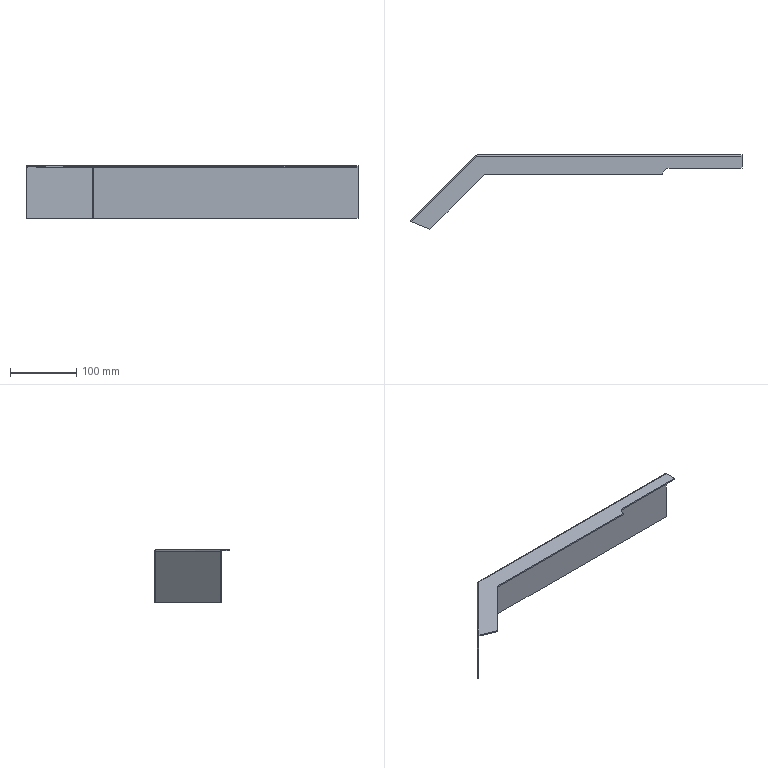Part | STEP file | Left Side Plate Filler Piece | 1 solid | 24 faces | box 502.056 x 112.482 x 80 mm | volume 112790 mm3 | plane 16 | cylinder 5 | spline 3 | commonest cylinder face diameters 1 x2 5 x2 20 x1
STEP:
#1=CARTESIAN_POINT('',(193.538,20.962,-2.5));
#2=VERTEX_POINT('',#1);
#3=CARTESIAN_POINT('',(-207.092,20.962,-2.5));
#4=VERTEX_POINT('',#3);
#5=CARTESIAN_POINT('',(0.,20.962,-2.5));
#6=DIRECTION('',(-1.,0.,0.));
#7=VECTOR('',#6,1000.);
#8=LINE('',#5,#7);
#9=EDGE_CURVE('',#2,#4,#8,.T.);
#10=ORIENTED_EDGE('',*,*,#9,.F.);
#11=CARTESIAN_POINT('',(193.538,20.962,-80.));
#12=VERTEX_POINT('',#11);
#13=CARTESIAN_POINT('',(193.538,20.962,0.));
#14=DIRECTION('',(0.,0.,1.));
#15=VECTOR('',#14,1000.);
#16=LINE('',#13,#15);
#17=EDGE_CURVE('',#12,#2,#16,.T.);
#18=ORIENTED_EDGE('',*,*,#17,.F.);
#19=CARTESIAN_POINT('',(-207.092,20.962,-80.));
#20=VERTEX_POINT('',#19);
#21=CARTESIAN_POINT('',(0.,20.962,-80.));
#22=DIRECTION('',(1.,0.,0.));
#23=VECTOR('',#22,1000.);
#24=LINE('',#21,#23);
#25=EDGE_CURVE('',#20,#12,#24,.T.);
#26=ORIENTED_EDGE('',*,*,#25,.F.);
#27=CARTESIAN_POINT('',(-207.092,20.962,0.));
#28=DIRECTION('',(0.,0.,-1.));
#29=VECTOR('',#28,1000.);
#30=LINE('',#27,#29);
#31=EDGE_CURVE('',#4,#20,#30,.T.);
#32=ORIENTED_EDGE('',*,*,#31,.F.);
#33=EDGE_LOOP('',(#10,#18,#26,#32));
#34=FACE_OUTER_BOUND('',#33,.T.);
#35=CARTESIAN_POINT('',(0.,20.962,0.));
#36=DIRECTION('',(0.,-1.,0.));
#37=DIRECTION('',(0.,0.,-1.));
#38=AXIS2_PLACEMENT_3D('',#35,#36,#37);
#39=PLANE('',#38);
#40=ADVANCED_FACE('',(#34),#39,.F.);
#41=CARTESIAN_POINT('',(-207.092,18.962,-80.));
#42=VERTEX_POINT('',#41);
#43=CARTESIAN_POINT('',(-207.092,18.962,-2.5));
#44=VERTEX_POINT('',#43);
#45=CARTESIAN_POINT('',(-207.092,18.962,-2.));
#46=DIRECTION('',(0.,0.,1.));
#47=VECTOR('',#46,1000.);
#48=LINE('',#45,#47);
#49=EDGE_CURVE('',#42,#44,#48,.T.);
#50=ORIENTED_EDGE('',*,*,#49,.T.);
#51=CARTESIAN_POINT('',(-207.092,18.962,-2.5));
#52=DIRECTION('',(0.,1.,0.));
#53=VECTOR('',#52,1000.);
#54=LINE('',#51,#53);
#55=EDGE_CURVE('',#44,#4,#54,.T.);
#56=ORIENTED_EDGE('',*,*,#55,.T.);
#57=ORIENTED_EDGE('',*,*,#31,.T.);
#58=CARTESIAN_POINT('',(-207.092,18.962,-80.));
#59=DIRECTION('',(0.,-1.,0.));
#60=VECTOR('',#59,1000.);
#61=LINE('',#58,#60);
#62=EDGE_CURVE('',#20,#42,#61,.T.);
#63=ORIENTED_EDGE('',*,*,#62,.T.);
#64=EDGE_LOOP('',(#50,#56,#57,#63));
#65=FACE_OUTER_BOUND('',#64,.T.);
#66=CARTESIAN_POINT('',(-207.092,18.962,-2.));
#67=DIRECTION('',(-1.,0.,0.));
#68=DIRECTION('',(0.,0.,1.));
#69=AXIS2_PLACEMENT_3D('',#66,#67,#68);
#70=PLANE('',#69);
#71=ADVANCED_FACE('',(#65),#70,.T.);
#72=ORIENTED_EDGE('',*,*,#9,.T.);
#73=CARTESIAN_POINT('',(-207.426,18.462,0.));
#74=VERTEX_POINT('',#73);
#75=CARTESIAN_POINT('',(-207.092,20.962,-2.5));
#76=CARTESIAN_POINT('',(-207.12,20.962,-2.173));
#77=CARTESIAN_POINT('',(-207.148,20.897,-1.846));
#78=CARTESIAN_POINT('',(-207.204,20.646,-1.241));
#79=CARTESIAN_POINT('',(-207.232,20.461,-0.9636));
#80=CARTESIAN_POINT('',(-207.287,19.998,-0.5008));
#81=CARTESIAN_POINT('',(-207.315,19.721,-0.3155));
#82=CARTESIAN_POINT('',(-207.371,19.116,-0.06507));
#83=CARTESIAN_POINT('',(-207.399,18.789,0.));
#84=CARTESIAN_POINT('',(-207.426,18.462,0.));
#85=B_SPLINE_CURVE_WITH_KNOTS('',3,(#75,#76,#77,#78,#79,#80,#81,#82,#83,#84),.UNSPECIFIED.,.F.,.F.,(4,2,2,2,4),(0.,0.25,0.5,0.75,1.),.UNSPECIFIED.);
#86=EDGE_CURVE('',#4,#74,#85,.T.);
#87=ORIENTED_EDGE('',*,*,#86,.T.);
#88=CARTESIAN_POINT('',(193.538,18.462,0.));
#89=VERTEX_POINT('',#88);
#90=CARTESIAN_POINT('',(193.538,18.462,0.));
#91=DIRECTION('',(1.,0.,0.));
#92=VECTOR('',#91,1000.);
#93=LINE('',#90,#92);
#94=EDGE_CURVE('',#74,#89,#93,.T.);
#95=ORIENTED_EDGE('',*,*,#94,.T.);
#96=CARTESIAN_POINT('',(193.538,18.462,-2.5));
#97=DIRECTION('',(-1.,0.,0.));
#98=DIRECTION('',(0.,0.,-1.));
#99=AXIS2_PLACEMENT_3D('',#96,#97,#98);
#100=CIRCLE('',#99,2.5);
#101=EDGE_CURVE('',#89,#2,#100,.T.);
#102=ORIENTED_EDGE('',*,*,#101,.T.);
#103=EDGE_LOOP('',(#72,#87,#95,#102));
#104=FACE_OUTER_BOUND('',#103,.T.);
#105=CARTESIAN_POINT('',(193.538,18.462,-2.5));
#106=DIRECTION('',(1.,0.,0.));
#107=DIRECTION('',(0.,0.,-1.));
#108=AXIS2_PLACEMENT_3D('',#105,#106,#107);
#109=CYLINDRICAL_SURFACE('',#108,2.5);
#110=ADVANCED_FACE('',(#104),#109,.T.);
#111=CARTESIAN_POINT('',(193.538,18.962,-80.));
#112=VERTEX_POINT('',#111);
#113=CARTESIAN_POINT('',(193.538,18.962,-2.5));
#114=VERTEX_POINT('',#113);
#115=CARTESIAN_POINT('',(193.538,18.962,-80.));
#116=DIRECTION('',(0.,0.,1.));
#117=VECTOR('',#116,1000.);
#118=LINE('',#115,#117);
#119=EDGE_CURVE('',#112,#114,#118,.T.);
#120=ORIENTED_EDGE('',*,*,#119,.F.);
#121=CARTESIAN_POINT('',(193.538,20.962,-80.));
#122=DIRECTION('',(0.,-1.,0.));
#123=VECTOR('',#122,1000.);
#124=LINE('',#121,#123);
#125=EDGE_CURVE('',#12,#112,#124,.T.);
#126=ORIENTED_EDGE('',*,*,#125,.F.);
#127=ORIENTED_EDGE('',*,*,#17,.T.);
#128=ORIENTED_EDGE('',*,*,#101,.F.);
#129=CARTESIAN_POINT('',(193.538,0.9619,0.));
#130=VERTEX_POINT('',#129);
#131=CARTESIAN_POINT('',(193.538,0.,0.));
#132=DIRECTION('',(0.,1.,0.));
#133=VECTOR('',#132,1000.);
#134=LINE('',#131,#133);
#135=EDGE_CURVE('',#130,#89,#134,.T.);
#136=ORIENTED_EDGE('',*,*,#135,.F.);
#137=CARTESIAN_POINT('',(193.538,0.9619,-2.));
#138=VERTEX_POINT('',#137);
#139=CARTESIAN_POINT('',(193.538,0.9619,-2.));
#140=DIRECTION('',(0.,0.,-1.));
#141=VECTOR('',#140,1000.);
#142=LINE('',#139,#141);
#143=EDGE_CURVE('',#130,#138,#142,.T.);
#144=ORIENTED_EDGE('',*,*,#143,.T.);
#145=CARTESIAN_POINT('',(193.538,18.462,-2.));
#146=VERTEX_POINT('',#145);
#147=CARTESIAN_POINT('',(193.538,-9.038,-2.));
#148=DIRECTION('',(0.,1.,0.));
#149=VECTOR('',#148,1000.);
#150=LINE('',#147,#149);
#151=EDGE_CURVE('',#138,#146,#150,.T.);
#152=ORIENTED_EDGE('',*,*,#151,.T.);
#153=CARTESIAN_POINT('',(193.538,18.462,-2.5));
#154=DIRECTION('',(1.,0.,0.));
#155=DIRECTION('',(0.,0.,-1.));
#156=AXIS2_PLACEMENT_3D('',#153,#154,#155);
#157=CIRCLE('',#156,0.5);
#158=EDGE_CURVE('',#114,#146,#157,.T.);
#159=ORIENTED_EDGE('',*,*,#158,.F.);
#160=EDGE_LOOP('',(#120,#126,#127,#128,#136,#144,#152,#159));
#161=FACE_OUTER_BOUND('',#160,.T.);
#162=CARTESIAN_POINT('',(193.538,20.962,-80.));
#163=DIRECTION('',(-1.,0.,0.));
#164=DIRECTION('',(0.,-1.,0.));
#165=AXIS2_PLACEMENT_3D('',#162,#163,#164);
#166=PLANE('',#165);
#167=ADVANCED_FACE('',(#161),#166,.F.);
#168=ORIENTED_EDGE('',*,*,#25,.T.);
#169=ORIENTED_EDGE('',*,*,#125,.T.);
#170=CARTESIAN_POINT('',(-208.462,18.962,-80.));
#171=DIRECTION('',(1.,0.,0.));
#172=VECTOR('',#171,1000.);
#173=LINE('',#170,#172);
#174=EDGE_CURVE('',#42,#112,#173,.T.);
#175=ORIENTED_EDGE('',*,*,#174,.F.);
#176=ORIENTED_EDGE('',*,*,#62,.F.);
#177=EDGE_LOOP('',(#168,#169,#175,#176));
#178=FACE_OUTER_BOUND('',#177,.T.);
#179=CARTESIAN_POINT('',(-208.462,20.962,-80.));
#180=DIRECTION('',(0.,0.,1.));
#181=DIRECTION('',(0.,-1.,0.));
#182=AXIS2_PLACEMENT_3D('',#179,#180,#181);
#183=PLANE('',#182);
#184=ADVANCED_FACE('',(#178),#183,.F.);
#185=CARTESIAN_POINT('',(-207.426,18.462,-2.));
#186=VERTEX_POINT('',#185);
#187=CARTESIAN_POINT('',(-207.092,18.962,-2.5));
#188=CARTESIAN_POINT('',(-207.148,18.962,-2.369));
#189=CARTESIAN_POINT('',(-207.204,18.908,-2.239));
#190=CARTESIAN_POINT('',(-207.315,18.723,-2.054));
#191=CARTESIAN_POINT('',(-207.371,18.593,-2.));
#192=CARTESIAN_POINT('',(-207.426,18.462,-2.));
#193=B_SPLINE_CURVE_WITH_KNOTS('',3,(#187,#188,#189,#190,#191,#192),.UNSPECIFIED.,.F.,.F.,(4,2,4),(0.,0.5,1.),.UNSPECIFIED.);
#194=EDGE_CURVE('',#44,#186,#193,.T.);
#195=ORIENTED_EDGE('',*,*,#194,.T.);
#196=CARTESIAN_POINT('',(-207.426,18.462,-1.));
#197=DIRECTION('',(0.,0.,-1.));
#198=VECTOR('',#197,1000.);
#199=LINE('',#196,#198);
#200=EDGE_CURVE('',#74,#186,#199,.T.);
#201=ORIENTED_EDGE('',*,*,#200,.F.);
#202=ORIENTED_EDGE('',*,*,#86,.F.);
#203=ORIENTED_EDGE('',*,*,#55,.F.);
#204=EDGE_LOOP('',(#195,#201,#202,#203));
#205=FACE_OUTER_BOUND('',#204,.T.);
#206=CARTESIAN_POINT('',(-207.426,18.462,0.02));
#207=CARTESIAN_POINT('',(-207.399,18.792,0.02));
#208=CARTESIAN_POINT('',(-207.371,19.122,-0.04559));
#209=CARTESIAN_POINT('',(-207.315,19.731,-0.2981));
#210=CARTESIAN_POINT('',(-207.287,20.011,-0.4848));
#211=CARTESIAN_POINT('',(-207.232,20.477,-0.9513));
#212=CARTESIAN_POINT('',(-207.204,20.664,-1.231));
#213=CARTESIAN_POINT('',(-207.148,20.916,-1.84));
#214=CARTESIAN_POINT('',(-207.12,20.982,-2.17));
#215=CARTESIAN_POINT('',(-207.092,20.982,-2.5));
#216=CARTESIAN_POINT('',(-207.426,18.462,0.));
#217=CARTESIAN_POINT('',(-207.399,18.789,0.));
#218=CARTESIAN_POINT('',(-207.371,19.116,-0.06507));
#219=CARTESIAN_POINT('',(-207.315,19.721,-0.3155));
#220=CARTESIAN_POINT('',(-207.287,19.998,-0.5008));
#221=CARTESIAN_POINT('',(-207.232,20.461,-0.9636));
#222=CARTESIAN_POINT('',(-207.204,20.646,-1.241));
#223=CARTESIAN_POINT('',(-207.148,20.897,-1.846));
#224=CARTESIAN_POINT('',(-207.12,20.962,-2.173));
#225=CARTESIAN_POINT('',(-207.092,20.962,-2.5));
#226=CARTESIAN_POINT('',(-207.426,18.462,-2.));
#227=CARTESIAN_POINT('',(-207.399,18.527,-2.));
#228=CARTESIAN_POINT('',(-207.371,18.593,-2.013));
#229=CARTESIAN_POINT('',(-207.315,18.714,-2.063));
#230=CARTESIAN_POINT('',(-207.287,18.769,-2.1));
#231=CARTESIAN_POINT('',(-207.232,18.862,-2.193));
#232=CARTESIAN_POINT('',(-207.204,18.899,-2.248));
#233=CARTESIAN_POINT('',(-207.148,18.949,-2.369));
#234=CARTESIAN_POINT('',(-207.12,18.962,-2.435));
#235=CARTESIAN_POINT('',(-207.092,18.962,-2.5));
#236=CARTESIAN_POINT('',(-207.426,18.462,-2.02));
#237=CARTESIAN_POINT('',(-207.399,18.525,-2.02));
#238=CARTESIAN_POINT('',(-207.371,18.588,-2.033));
#239=CARTESIAN_POINT('',(-207.315,18.704,-2.081));
#240=CARTESIAN_POINT('',(-207.287,18.757,-2.116));
#241=CARTESIAN_POINT('',(-207.232,18.846,-2.205));
#242=CARTESIAN_POINT('',(-207.204,18.881,-2.258));
#243=CARTESIAN_POINT('',(-207.148,18.929,-2.374));
#244=CARTESIAN_POINT('',(-207.12,18.942,-2.437));
#245=CARTESIAN_POINT('',(-207.092,18.942,-2.5));
#246=B_SPLINE_SURFACE_WITH_KNOTS('',1,3,((#206,#207,#208,#209,#210,#211,#212,#213,#214,#215),(#216,#217,#218,#219,#220,#221,#222,#223,#224,#225),(#226,#227,#228,#229,#230,#231,#232,#233,#234,#235),(#236,#237,#238,#239,#240,#241,#242,#243,#244,#245)),.UNSPECIFIED.,.F.,.F.,.F.,(2,1,1,2),(4,2,2,2,4),(-0.01,0.,1.,1.01),(0.,0.25,0.5,0.75,1.),.UNSPECIFIED.);
#247=ADVANCED_FACE('',(#205),#246,.F.);
#248=ORIENTED_EDGE('',*,*,#174,.T.);
#249=ORIENTED_EDGE('',*,*,#119,.T.);
#250=CARTESIAN_POINT('',(0.,18.962,-2.5));
#251=DIRECTION('',(-1.,0.,0.));
#252=VECTOR('',#251,1000.);
#253=LINE('',#250,#252);
#254=EDGE_CURVE('',#114,#44,#253,.T.);
#255=ORIENTED_EDGE('',*,*,#254,.T.);
#256=ORIENTED_EDGE('',*,*,#49,.F.);
#257=EDGE_LOOP('',(#248,#249,#255,#256));
#258=FACE_OUTER_BOUND('',#257,.T.);
#259=CARTESIAN_POINT('',(0.,18.962,0.));
#260=DIRECTION('',(0.,-1.,0.));
#261=DIRECTION('',(0.,0.,-1.));
#262=AXIS2_PLACEMENT_3D('',#259,#260,#261);
#263=PLANE('',#262);
#264=ADVANCED_FACE('',(#258),#263,.T.);
#265=CARTESIAN_POINT('',(-306.018,-80.129,0.));
#266=VERTEX_POINT('',#265);
#267=CARTESIAN_POINT('',(-278.518,-91.52,0.));
#268=VERTEX_POINT('',#267);
#269=CARTESIAN_POINT('',(-306.018,-80.129,0.));
#270=DIRECTION('',(0.9239,-0.3827,0.));
#271=VECTOR('',#270,1000.);
#272=LINE('',#269,#271);
#273=EDGE_CURVE('',#266,#268,#272,.T.);
#274=ORIENTED_EDGE('',*,*,#273,.T.);
#275=CARTESIAN_POINT('',(-196.036,-9.038,0.));
#276=VERTEX_POINT('',#275);
#277=CARTESIAN_POINT('',(-278.518,-91.52,0.));
#278=DIRECTION('',(0.7071,0.7071,0.));
#279=VECTOR('',#278,1000.);
#280=LINE('',#277,#279);
#281=EDGE_CURVE('',#268,#276,#280,.T.);
#282=ORIENTED_EDGE('',*,*,#281,.T.);
#283=CARTESIAN_POINT('',(73.538,-9.038,0.));
#284=VERTEX_POINT('',#283);
#285=CARTESIAN_POINT('',(0.,-9.038,0.));
#286=DIRECTION('',(1.,0.,0.));
#287=VECTOR('',#286,1000.);
#288=LINE('',#285,#287);
#289=EDGE_CURVE('',#276,#284,#288,.T.);
#290=ORIENTED_EDGE('',*,*,#289,.T.);
#291=CARTESIAN_POINT('',(83.538,0.9619,0.));
#292=VERTEX_POINT('',#291);
#293=CARTESIAN_POINT('',(83.538,-9.038,0.));
#294=DIRECTION('',(0.,0.,-1.));
#295=DIRECTION('',(-1.,0.,0.));
#296=AXIS2_PLACEMENT_3D('',#293,#294,#295);
#297=CIRCLE('',#296,10.);
#298=EDGE_CURVE('',#284,#292,#297,.T.);
#299=ORIENTED_EDGE('',*,*,#298,.T.);
#300=CARTESIAN_POINT('',(0.,0.9619,0.));
#301=DIRECTION('',(1.,0.,0.));
#302=VECTOR('',#301,1000.);
#303=LINE('',#300,#302);
#304=EDGE_CURVE('',#292,#130,#303,.T.);
#305=ORIENTED_EDGE('',*,*,#304,.T.);
#306=ORIENTED_EDGE('',*,*,#135,.T.);
#307=ORIENTED_EDGE('',*,*,#94,.F.);
#308=CARTESIAN_POINT('',(-207.426,18.462,0.));
#309=DIRECTION('',(-0.7071,-0.7071,0.));
#310=VECTOR('',#309,1000.);
#311=LINE('',#308,#310);
#312=EDGE_CURVE('',#74,#266,#311,.T.);
#313=ORIENTED_EDGE('',*,*,#312,.T.);
#314=EDGE_LOOP('',(#274,#282,#290,#299,#305,#306,#307,#313));
#315=FACE_OUTER_BOUND('',#314,.T.);
#316=CARTESIAN_POINT('',(0.,0.,0.));
#317=DIRECTION('',(0.,0.,1.));
#318=DIRECTION('',(1.,0.,0.));
#319=AXIS2_PLACEMENT_3D('',#316,#317,#318);
#320=PLANE('',#319);
#321=ADVANCED_FACE('',(#315),#320,.T.);
#322=CARTESIAN_POINT('',(-209.43,19.993,-2.5));
#323=VERTEX_POINT('',#322);
#324=CARTESIAN_POINT('',(-208.016,18.579,-2.5));
#325=VERTEX_POINT('',#324);
#326=CARTESIAN_POINT('',(-208.723,19.286,-2.5));
#327=DIRECTION('',(0.7071,-0.7071,0.));
#328=VECTOR('',#327,1000.);
#329=LINE('',#326,#328);
#330=EDGE_CURVE('',#323,#325,#329,.T.);
#331=ORIENTED_EDGE('',*,*,#330,.F.);
#332=CARTESIAN_POINT('',(-207.426,18.462,0.));
#333=CARTESIAN_POINT('',(-207.677,18.674,0.));
#334=CARTESIAN_POINT('',(-207.928,18.885,-0.06507));
#335=CARTESIAN_POINT('',(-208.395,19.273,-0.3155));
#336=CARTESIAN_POINT('',(-208.611,19.45,-0.5008));
#337=CARTESIAN_POINT('',(-208.978,19.738,-0.9636));
#338=CARTESIAN_POINT('',(-209.129,19.849,-1.241));
#339=CARTESIAN_POINT('',(-209.345,19.987,-1.846));
#340=CARTESIAN_POINT('',(-209.411,20.013,-2.173));
#341=CARTESIAN_POINT('',(-209.43,19.993,-2.5));
#342=B_SPLINE_CURVE_WITH_KNOTS('',3,(#332,#333,#334,#335,#336,#337,#338,#339,#340,#341),.UNSPECIFIED.,.F.,.F.,(4,2,2,2,4),(0.,0.25,0.5,0.75,1.),.UNSPECIFIED.);
#343=EDGE_CURVE('',#74,#323,#342,.T.);
#344=ORIENTED_EDGE('',*,*,#343,.F.);
#345=ORIENTED_EDGE('',*,*,#200,.T.);
#346=CARTESIAN_POINT('',(-207.426,18.462,-2.));
#347=CARTESIAN_POINT('',(-207.558,18.515,-2.));
#348=CARTESIAN_POINT('',(-207.69,18.568,-2.054));
#349=CARTESIAN_POINT('',(-207.899,18.62,-2.239));
#350=CARTESIAN_POINT('',(-207.977,18.619,-2.369));
#351=CARTESIAN_POINT('',(-208.016,18.579,-2.5));
#352=B_SPLINE_CURVE_WITH_KNOTS('',3,(#346,#347,#348,#349,#350,#351),.UNSPECIFIED.,.F.,.F.,(4,2,4),(0.,0.5,1.),.UNSPECIFIED.);
#353=EDGE_CURVE('',#186,#325,#352,.T.);
#354=ORIENTED_EDGE('',*,*,#353,.T.);
#355=EDGE_LOOP('',(#331,#344,#345,#354));
#356=FACE_OUTER_BOUND('',#355,.T.);
#357=CARTESIAN_POINT('',(-209.445,20.008,-2.5));
#358=CARTESIAN_POINT('',(-209.425,20.027,-2.17));
#359=CARTESIAN_POINT('',(-209.359,20.001,-1.84));
#360=CARTESIAN_POINT('',(-209.141,19.861,-1.231));
#361=CARTESIAN_POINT('',(-208.989,19.749,-0.9513));
#362=CARTESIAN_POINT('',(-208.62,19.459,-0.4848));
#363=CARTESIAN_POINT('',(-208.403,19.281,-0.2981));
#364=CARTESIAN_POINT('',(-207.932,18.889,-0.04559));
#365=CARTESIAN_POINT('',(-207.679,18.676,0.02));
#366=CARTESIAN_POINT('',(-207.426,18.462,0.02));
#367=CARTESIAN_POINT('',(-209.43,19.993,-2.5));
#368=CARTESIAN_POINT('',(-209.411,20.013,-2.173));
#369=CARTESIAN_POINT('',(-209.345,19.987,-1.846));
#370=CARTESIAN_POINT('',(-209.129,19.849,-1.241));
#371=CARTESIAN_POINT('',(-208.978,19.738,-0.9636));
#372=CARTESIAN_POINT('',(-208.611,19.45,-0.5008));
#373=CARTESIAN_POINT('',(-208.395,19.273,-0.3155));
#374=CARTESIAN_POINT('',(-207.928,18.885,-0.06507));
#375=CARTESIAN_POINT('',(-207.678,18.674,0.));
#376=CARTESIAN_POINT('',(-207.426,18.462,0.));
#377=CARTESIAN_POINT('',(-208.016,18.579,-2.5));
#378=CARTESIAN_POINT('',(-207.997,18.599,-2.435));
#379=CARTESIAN_POINT('',(-207.968,18.609,-2.369));
#380=CARTESIAN_POINT('',(-207.893,18.613,-2.248));
#381=CARTESIAN_POINT('',(-207.847,18.607,-2.193));
#382=CARTESIAN_POINT('',(-207.742,18.581,-2.1));
#383=CARTESIAN_POINT('',(-207.683,18.561,-2.063));
#384=CARTESIAN_POINT('',(-207.558,18.515,-2.013));
#385=CARTESIAN_POINT('',(-207.492,18.489,-2.));
#386=CARTESIAN_POINT('',(-207.426,18.462,-2.));
#387=CARTESIAN_POINT('',(-208.002,18.565,-2.5));
#388=CARTESIAN_POINT('',(-207.982,18.585,-2.437));
#389=CARTESIAN_POINT('',(-207.954,18.596,-2.374));
#390=CARTESIAN_POINT('',(-207.88,18.601,-2.258));
#391=CARTESIAN_POINT('',(-207.836,18.595,-2.205));
#392=CARTESIAN_POINT('',(-207.733,18.572,-2.116));
#393=CARTESIAN_POINT('',(-207.676,18.554,-2.081));
#394=CARTESIAN_POINT('',(-207.555,18.511,-2.033));
#395=CARTESIAN_POINT('',(-207.491,18.487,-2.02));
#396=CARTESIAN_POINT('',(-207.426,18.462,-2.02));
#397=B_SPLINE_SURFACE_WITH_KNOTS('',1,3,((#357,#358,#359,#360,#361,#362,#363,#364,#365,#366),(#367,#368,#369,#370,#371,#372,#373,#374,#375,#376),(#377,#378,#379,#380,#381,#382,#383,#384,#385,#386),(#387,#388,#389,#390,#391,#392,#393,#394,#395,#396)),.UNSPECIFIED.,.F.,.F.,.F.,(2,1,1,2),(4,2,2,2,4),(-0.01,0.,1.,1.01),(0.,0.25,0.5,0.75,1.),.UNSPECIFIED.);
#398=ADVANCED_FACE('',(#356),#397,.F.);
#399=ORIENTED_EDGE('',*,*,#194,.F.);
#400=ORIENTED_EDGE('',*,*,#254,.F.);
#401=ORIENTED_EDGE('',*,*,#158,.T.);
#402=CARTESIAN_POINT('',(193.538,18.462,-2.));
#403=DIRECTION('',(1.,0.,0.));
#404=VECTOR('',#403,1000.);
#405=LINE('',#402,#404);
#406=EDGE_CURVE('',#186,#146,#405,.T.);
#407=ORIENTED_EDGE('',*,*,#406,.F.);
#408=EDGE_LOOP('',(#399,#400,#401,#407));
#409=FACE_OUTER_BOUND('',#408,.T.);
#410=CARTESIAN_POINT('',(193.538,18.462,-2.5));
#411=DIRECTION('',(1.,0.,0.));
#412=DIRECTION('',(0.,0.,-1.));
#413=AXIS2_PLACEMENT_3D('',#410,#411,#412);
#414=CYLINDRICAL_SURFACE('',#413,0.5);
#415=ADVANCED_FACE('',(#409),#414,.F.);
#416=CARTESIAN_POINT('',(-278.518,-91.52,-2.));
#417=VERTEX_POINT('',#416);
#418=CARTESIAN_POINT('',(-196.036,-9.038,-2.));
#419=VERTEX_POINT('',#418);
#420=CARTESIAN_POINT('',(-278.518,-91.52,-2.));
#421=DIRECTION('',(0.7071,0.7071,0.));
#422=VECTOR('',#421,1000.);
#423=LINE('',#420,#422);
#424=EDGE_CURVE('',#417,#419,#423,.T.);
#425=ORIENTED_EDGE('',*,*,#424,.T.);
#426=CARTESIAN_POINT('',(-196.036,-9.038,-2.));
#427=DIRECTION('',(0.,0.,1.));
#428=VECTOR('',#427,1000.);
#429=LINE('',#426,#428);
#430=EDGE_CURVE('',#419,#276,#429,.T.);
#431=ORIENTED_EDGE('',*,*,#430,.T.);
#432=ORIENTED_EDGE('',*,*,#281,.F.);
#433=CARTESIAN_POINT('',(-278.518,-91.52,-2.));
#434=DIRECTION('',(0.,0.,-1.));
#435=VECTOR('',#434,1000.);
#436=LINE('',#433,#435);
#437=EDGE_CURVE('',#268,#417,#436,.T.);
#438=ORIENTED_EDGE('',*,*,#437,.T.);
#439=EDGE_LOOP('',(#425,#431,#432,#438));
#440=FACE_OUTER_BOUND('',#439,.T.);
#441=CARTESIAN_POINT('',(-278.518,-91.52,-2.));
#442=DIRECTION('',(0.7071,-0.7071,0.));
#443=DIRECTION('',(0.7071,0.7071,0.));
#444=AXIS2_PLACEMENT_3D('',#441,#442,#443);
#445=PLANE('',#444);
#446=ADVANCED_FACE('',(#440),#445,.T.);
#447=CARTESIAN_POINT('',(-306.018,-80.129,-2.));
#448=VERTEX_POINT('',#447);
#449=CARTESIAN_POINT('',(-308.518,-79.094,-2.));
#450=DIRECTION('',(0.9239,-0.3827,0.));
#451=VECTOR('',#450,1000.);
#452=LINE('',#449,#451);
#453=EDGE_CURVE('',#448,#417,#452,.T.);
#454=ORIENTED_EDGE('',*,*,#453,.T.);
#455=ORIENTED_EDGE('',*,*,#437,.F.);
#456=ORIENTED_EDGE('',*,*,#273,.F.);
#457=CARTESIAN_POINT('',(-306.018,-80.129,-2.));
#458=DIRECTION('',(0.,0.,-1.));
#459=VECTOR('',#458,1000.);
#460=LINE('',#457,#459);
#461=EDGE_CURVE('',#266,#448,#460,.T.);
#462=ORIENTED_EDGE('',*,*,#461,.T.);
#463=EDGE_LOOP('',(#454,#455,#456,#462));
#464=FACE_OUTER_BOUND('',#463,.T.);
#465=CARTESIAN_POINT('',(-308.518,-79.094,-2.));
#466=DIRECTION('',(-0.3827,-0.9239,0.));
#467=DIRECTION('',(0.9239,-0.3827,0.));
#468=AXIS2_PLACEMENT_3D('',#465,#466,#467);
#469=PLANE('',#468);
#470=ADVANCED_FACE('',(#464),#469,.T.);
#471=CARTESIAN_POINT('',(-308.518,-79.094,-2.5));
#472=VERTEX_POINT('',#471);
#473=CARTESIAN_POINT('',(-209.194,20.23,-2.5));
#474=DIRECTION('',(-0.7071,-0.7071,0.));
#475=VECTOR('',#474,1000.);
#476=LINE('',#473,#475);
#477=EDGE_CURVE('',#323,#472,#476,.T.);
#478=ORIENTED_EDGE('',*,*,#477,.T.);
#479=CARTESIAN_POINT('',(-308.518,-79.094,-2.5));
#480=CARTESIAN_POINT('',(-308.456,-79.032,-2.17));
#481=CARTESIAN_POINT('',(-308.352,-79.017,-1.851));
#482=CARTESIAN_POINT('',(-308.051,-79.072,-1.242));
#483=CARTESIAN_POINT('',(-307.861,-79.141,-0.967));
#484=CARTESIAN_POINT('',(-307.523,-79.296,-0.6175));
#485=CARTESIAN_POINT('',(-307.403,-79.355,-0.514));
#486=CARTESIAN_POINT('',(-307.151,-79.486,-0.3324));
#487=CARTESIAN_POINT('',(-307.016,-79.558,-0.2538));
#488=CARTESIAN_POINT('',(-306.741,-79.711,-0.1283));
#489=CARTESIAN_POINT('',(-306.601,-79.791,-0.08082));
#490=CARTESIAN_POINT('',(-306.313,-79.957,-0.01658));
#491=CARTESIAN_POINT('',(-306.165,-80.043,0.));
#492=CARTESIAN_POINT('',(-306.018,-80.129,0.));
#493=B_SPLINE_CURVE_WITH_KNOTS('',3,(#479,#480,#481,#482,#483,#484,#485,#486,#487,#488,#489,#490,#491,#492),.UNSPECIFIED.,.F.,.F.,(4,2,2,2,2,2,4),(0.,0.001005,0.002011,0.002514,0.003016,0.003519,0.004022),.UNSPECIFIED.);
#494=EDGE_CURVE('',#472,#266,#493,.T.);
#495=ORIENTED_EDGE('',*,*,#494,.T.);
#496=ORIENTED_EDGE('',*,*,#312,.F.);
#497=ORIENTED_EDGE('',*,*,#343,.T.);
#498=EDGE_LOOP('',(#478,#495,#496,#497));
#499=FACE_OUTER_BOUND('',#498,.T.);
#500=CARTESIAN_POINT('',(-207.426,18.462,-2.5));
#501=DIRECTION('',(0.7071,0.7071,0.));
#502=DIRECTION('',(-0.7071,0.7071,0.));
#503=AXIS2_PLACEMENT_3D('',#500,#501,#502);
#504=CYLINDRICAL_SURFACE('',#503,2.5);
#505=ADVANCED_FACE('',(#499),#504,.T.);
#506=CARTESIAN_POINT('',(83.538,0.9619,-2.));
#507=VERTEX_POINT('',#506);
#508=CARTESIAN_POINT('',(83.538,0.9619,-10.));
#509=DIRECTION('',(0.,0.,1.));
#510=VECTOR('',#509,1000.);
#511=LINE('',#508,#510);
#512=EDGE_CURVE('',#507,#292,#511,.T.);
#513=ORIENTED_EDGE('',*,*,#512,.F.);
#514=CARTESIAN_POINT('',(193.538,0.9619,-2.));
#515=DIRECTION('',(-1.,0.,0.));
#516=VECTOR('',#515,1000.);
#517=LINE('',#514,#516);
#518=EDGE_CURVE('',#138,#507,#517,.T.);
#519=ORIENTED_EDGE('',*,*,#518,.F.);
#520=ORIENTED_EDGE('',*,*,#143,.F.);
#521=ORIENTED_EDGE('',*,*,#304,.F.);
#522=EDGE_LOOP('',(#513,#519,#520,#521));
#523=FACE_OUTER_BOUND('',#522,.T.);
#524=CARTESIAN_POINT('',(193.538,0.9619,-10.));
#525=DIRECTION('',(0.,1.,0.));
#526=DIRECTION('',(-1.,0.,0.));
#527=AXIS2_PLACEMENT_3D('',#524,#525,#526);
#528=PLANE('',#527);
#529=ADVANCED_FACE('',(#523),#528,.F.);
#530=ORIENTED_EDGE('',*,*,#512,.T.);
#531=ORIENTED_EDGE('',*,*,#298,.F.);
#532=CARTESIAN_POINT('',(73.538,-9.038,-2.));
#533=VERTEX_POINT('',#532);
#534=CARTESIAN_POINT('',(73.538,-9.038,-10.));
#535=DIRECTION('',(0.,0.,1.));
#536=VECTOR('',#535,1000.);
#537=LINE('',#534,#536);
#538=EDGE_CURVE('',#533,#284,#537,.T.);
#539=ORIENTED_EDGE('',*,*,#538,.F.);
#540=CARTESIAN_POINT('',(83.538,-9.038,-2.));
#541=DIRECTION('',(0.,0.,1.));
#542=DIRECTION('',(-1.,0.,0.));
#543=AXIS2_PLACEMENT_3D('',#540,#541,#542);
#544=CIRCLE('',#543,10.);
#545=EDGE_CURVE('',#507,#533,#544,.T.);
#546=ORIENTED_EDGE('',*,*,#545,.F.);
#547=EDGE_LOOP('',(#530,#531,#539,#546));
#548=FACE_OUTER_BOUND('',#547,.T.);
#549=CARTESIAN_POINT('',(83.538,-9.038,-10.));
#550=DIRECTION('',(0.,0.,-1.));
#551=DIRECTION('',(-1.,0.,0.));
#552=AXIS2_PLACEMENT_3D('',#549,#550,#551);
#553=CYLINDRICAL_SURFACE('',#552,10.);
#554=ADVANCED_FACE('',(#548),#553,.F.);
#555=ORIENTED_EDGE('',*,*,#430,.F.);
#556=CARTESIAN_POINT('',(-196.036,-9.038,-2.));
#557=DIRECTION('',(1.,0.,0.));
#558=VECTOR('',#557,1000.);
#559=LINE('',#556,#558);
#560=EDGE_CURVE('',#419,#533,#559,.T.);
#561=ORIENTED_EDGE('',*,*,#560,.T.);
#562=ORIENTED_EDGE('',*,*,#538,.T.);
#563=ORIENTED_EDGE('',*,*,#289,.F.);
#564=EDGE_LOOP('',(#555,#561,#562,#563));
#565=FACE_OUTER_BOUND('',#564,.T.);
#566=CARTESIAN_POINT('',(-196.036,-9.038,-2.));
#567=DIRECTION('',(0.,-1.,0.));
#568=DIRECTION('',(1.,0.,0.));
#569=AXIS2_PLACEMENT_3D('',#566,#567,#568);
#570=PLANE('',#569);
#571=ADVANCED_FACE('',(#565),#570,.T.);
#572=CARTESIAN_POINT('',(-209.43,19.993,-80.));
#573=VERTEX_POINT('',#572);
#574=CARTESIAN_POINT('',(-209.43,19.993,-2.));
#575=DIRECTION('',(0.,0.,-1.));
#576=VECTOR('',#575,1000.);
#577=LINE('',#574,#576);
#578=EDGE_CURVE('',#323,#573,#577,.T.);
#579=ORIENTED_EDGE('',*,*,#578,.F.);
#580=ORIENTED_EDGE('',*,*,#330,.T.);
#581=CARTESIAN_POINT('',(-208.016,18.579,-80.));
#582=VERTEX_POINT('',#581);
#583=CARTESIAN_POINT('',(-208.016,18.579,-2.));
#584=DIRECTION('',(0.,0.,1.));
#585=VECTOR('',#584,1000.);
#586=LINE('',#583,#585);
#587=EDGE_CURVE('',#582,#325,#586,.T.);
#588=ORIENTED_EDGE('',*,*,#587,.F.);
#589=CARTESIAN_POINT('',(-208.016,18.579,-80.));
#590=DIRECTION('',(0.7071,-0.7071,0.));
#591=VECTOR('',#590,1000.);
#592=LINE('',#589,#591);
#593=EDGE_CURVE('',#573,#582,#592,.T.);
#594=ORIENTED_EDGE('',*,*,#593,.F.);
#595=EDGE_LOOP('',(#579,#580,#588,#594));
#596=FACE_OUTER_BOUND('',#595,.T.);
#597=CARTESIAN_POINT('',(-208.016,18.579,-2.));
#598=DIRECTION('',(-0.7071,-0.7071,0.));
#599=DIRECTION('',(0.7071,-0.7071,0.));
#600=AXIS2_PLACEMENT_3D('',#597,#598,#599);
#601=PLANE('',#600);
#602=ADVANCED_FACE('',(#596),#601,.F.);
#603=ORIENTED_EDGE('',*,*,#545,.T.);
#604=ORIENTED_EDGE('',*,*,#560,.F.);
#605=ORIENTED_EDGE('',*,*,#424,.F.);
#606=ORIENTED_EDGE('',*,*,#453,.F.);
#607=CARTESIAN_POINT('',(-207.426,18.462,-2.));
#608=DIRECTION('',(-0.7071,-0.7071,0.));
#609=VECTOR('',#608,1000.);
#610=LINE('',#607,#609);
#611=EDGE_CURVE('',#186,#448,#610,.T.);
#612=ORIENTED_EDGE('',*,*,#611,.F.);
#613=ORIENTED_EDGE('',*,*,#406,.T.);
#614=ORIENTED_EDGE('',*,*,#151,.F.);
#615=ORIENTED_EDGE('',*,*,#518,.T.);
#616=EDGE_LOOP('',(#603,#604,#605,#606,#612,#613,#614,#615));
#617=FACE_OUTER_BOUND('',#616,.T.);
#618=CARTESIAN_POINT('',(0.,0.,-2.));
#619=DIRECTION('',(0.,0.,1.));
#620=DIRECTION('',(1.,0.,0.));
#621=AXIS2_PLACEMENT_3D('',#618,#619,#620);
#622=PLANE('',#621);
#623=ADVANCED_FACE('',(#617),#622,.F.);
#624=CARTESIAN_POINT('',(-307.103,-80.508,-2.5));
#625=VERTEX_POINT('',#624);
#626=CARTESIAN_POINT('',(-306.018,-80.129,-2.));
#627=CARTESIAN_POINT('',(-306.126,-80.144,-2.));
#628=CARTESIAN_POINT('',(-306.232,-80.159,-2.013));
#629=CARTESIAN_POINT('',(-306.439,-80.195,-2.063));
#630=CARTESIAN_POINT('',(-306.54,-80.217,-2.1));
#631=CARTESIAN_POINT('',(-306.82,-80.301,-2.238));
#632=CARTESIAN_POINT('',(-306.98,-80.385,-2.368));
#633=CARTESIAN_POINT('',(-307.103,-80.508,-2.5));
#634=B_SPLINE_CURVE_WITH_KNOTS('',3,(#626,#627,#628,#629,#630,#631,#632,#633),.UNSPECIFIED.,.F.,.F.,(4,2,2,4),(0.,0.0003231,0.0006462,0.001292),.UNSPECIFIED.);
#635=EDGE_CURVE('',#448,#625,#634,.T.);
#636=ORIENTED_EDGE('',*,*,#635,.F.);
#637=ORIENTED_EDGE('',*,*,#461,.F.);
#638=ORIENTED_EDGE('',*,*,#494,.F.);
#639=CARTESIAN_POINT('',(-307.81,-79.801,-2.5));
#640=DIRECTION('',(-0.7071,0.7071,0.));
#641=VECTOR('',#640,1000.);
#642=LINE('',#639,#641);
#643=EDGE_CURVE('',#625,#472,#642,.T.);
#644=ORIENTED_EDGE('',*,*,#643,.F.);
#645=EDGE_LOOP('',(#636,#637,#638,#644));
#646=FACE_OUTER_BOUND('',#645,.T.);
#647=CARTESIAN_POINT('',(-306.018,-80.129,0.02));
#648=CARTESIAN_POINT('',(-306.312,-79.957,0.02));
#649=CARTESIAN_POINT('',(-306.606,-79.785,-0.04559));
#650=CARTESIAN_POINT('',(-307.159,-79.476,-0.2981));
#651=CARTESIAN_POINT('',(-307.418,-79.339,-0.4848));
#652=CARTESIAN_POINT('',(-307.87,-79.131,-0.9513));
#653=CARTESIAN_POINT('',(-308.063,-79.06,-1.231));
#654=CARTESIAN_POINT('',(-308.363,-79.004,-1.84));
#655=CARTESIAN_POINT('',(-308.471,-79.018,-2.17));
#656=CARTESIAN_POINT('',(-308.532,-79.08,-2.5));
#657=CARTESIAN_POINT('',(-306.018,-80.129,0.));
#658=CARTESIAN_POINT('',(-306.31,-79.959,0.));
#659=CARTESIAN_POINT('',(-306.602,-79.789,-0.06507));
#660=CARTESIAN_POINT('',(-307.152,-79.483,-0.3155));
#661=CARTESIAN_POINT('',(-307.409,-79.348,-0.5008));
#662=CARTESIAN_POINT('',(-307.858,-79.143,-0.9636));
#663=CARTESIAN_POINT('',(-308.05,-79.073,-1.241));
#664=CARTESIAN_POINT('',(-308.35,-79.018,-1.846));
#665=CARTESIAN_POINT('',(-308.457,-79.033,-2.173));
#666=CARTESIAN_POINT('',(-308.518,-79.094,-2.5));
#667=CARTESIAN_POINT('',(-306.018,-80.129,-2.));
#668=CARTESIAN_POINT('',(-306.125,-80.144,-2.));
#669=CARTESIAN_POINT('',(-306.232,-80.159,-2.013));
#670=CARTESIAN_POINT('',(-306.44,-80.195,-2.063));
#671=CARTESIAN_POINT('',(-306.54,-80.217,-2.1));
#672=CARTESIAN_POINT('',(-306.727,-80.274,-2.193));
#673=CARTESIAN_POINT('',(-306.815,-80.308,-2.248));
#674=CARTESIAN_POINT('',(-306.972,-80.395,-2.369));
#675=CARTESIAN_POINT('',(-307.042,-80.447,-2.435));
#676=CARTESIAN_POINT('',(-307.103,-80.508,-2.5));
#677=CARTESIAN_POINT('',(-306.018,-80.129,-2.02));
#678=CARTESIAN_POINT('',(-306.123,-80.146,-2.02));
#679=CARTESIAN_POINT('',(-306.228,-80.162,-2.033));
#680=CARTESIAN_POINT('',(-306.432,-80.202,-2.081));
#681=CARTESIAN_POINT('',(-306.531,-80.226,-2.116));
#682=CARTESIAN_POINT('',(-306.716,-80.285,-2.205));
#683=CARTESIAN_POINT('',(-306.802,-80.321,-2.258));
#684=CARTESIAN_POINT('',(-306.958,-80.409,-2.374));
#685=CARTESIAN_POINT('',(-307.028,-80.461,-2.437));
#686=CARTESIAN_POINT('',(-307.089,-80.522,-2.5));
#687=B_SPLINE_SURFACE_WITH_KNOTS('',1,3,((#647,#648,#649,#650,#651,#652,#653,#654,#655,#656),(#657,#658,#659,#660,#661,#662,#663,#664,#665,#666),(#667,#668,#669,#670,#671,#672,#673,#674,#675,#676),(#677,#678,#679,#680,#681,#682,#683,#684,#685,#686)),.UNSPECIFIED.,.F.,.F.,.F.,(2,1,1,2),(4,2,2,2,4),(-0.01,0.,1.,1.01),(0.,0.25,0.5,0.75,1.),.UNSPECIFIED.);
#688=ADVANCED_FACE('',(#646),#687,.F.);
#689=ORIENTED_EDGE('',*,*,#578,.T.);
#690=CARTESIAN_POINT('',(-308.518,-79.094,-80.));
#691=VERTEX_POINT('',#690);
#692=CARTESIAN_POINT('',(-114.712,114.712,-80.));
#693=DIRECTION('',(0.7071,0.7071,0.));
#694=VECTOR('',#693,1000.);
#695=LINE('',#692,#694);
#696=EDGE_CURVE('',#691,#573,#695,.T.);
#697=ORIENTED_EDGE('',*,*,#696,.F.);
#698=CARTESIAN_POINT('',(-308.518,-79.094,0.));
#699=DIRECTION('',(0.,0.,-1.));
#700=VECTOR('',#699,1000.);
#701=LINE('',#698,#700);
#702=EDGE_CURVE('',#472,#691,#701,.T.);
#703=ORIENTED_EDGE('',*,*,#702,.F.);
#704=ORIENTED_EDGE('',*,*,#477,.F.);
#705=EDGE_LOOP('',(#689,#697,#703,#704));
#706=FACE_OUTER_BOUND('',#705,.T.);
#707=CARTESIAN_POINT('',(-114.712,114.712,0.));
#708=DIRECTION('',(0.7071,-0.7071,0.));
#709=DIRECTION('',(0.7071,0.7071,0.));
#710=AXIS2_PLACEMENT_3D('',#707,#708,#709);
#711=PLANE('',#710);
#712=ADVANCED_FACE('',(#706),#711,.F.);
#713=ORIENTED_EDGE('',*,*,#593,.T.);
#714=CARTESIAN_POINT('',(-307.103,-80.508,-80.));
#715=VERTEX_POINT('',#714);
#716=CARTESIAN_POINT('',(-307.103,-80.508,-80.));
#717=DIRECTION('',(0.7071,0.7071,0.));
#718=VECTOR('',#717,1000.);
#719=LINE('',#716,#718);
#720=EDGE_CURVE('',#715,#582,#719,.T.);
#721=ORIENTED_EDGE('',*,*,#720,.F.);
#722=CARTESIAN_POINT('',(-308.518,-79.094,-80.));
#723=DIRECTION('',(0.7071,-0.7071,0.));
#724=VECTOR('',#723,1000.);
#725=LINE('',#722,#724);
#726=EDGE_CURVE('',#691,#715,#725,.T.);
#727=ORIENTED_EDGE('',*,*,#726,.F.);
#728=ORIENTED_EDGE('',*,*,#696,.T.);
#729=EDGE_LOOP('',(#713,#721,#727,#728));
#730=FACE_OUTER_BOUND('',#729,.T.);
#731=CARTESIAN_POINT('',(-308.518,-79.094,-80.));
#732=DIRECTION('',(0.,0.,1.));
#733=DIRECTION('',(1.,0.,0.));
#734=AXIS2_PLACEMENT_3D('',#731,#732,#733);
#735=PLANE('',#734);
#736=ADVANCED_FACE('',(#730),#735,.F.);
#737=CARTESIAN_POINT('',(-307.103,-80.508,0.));
#738=DIRECTION('',(0.,0.,-1.));
#739=VECTOR('',#738,1000.);
#740=LINE('',#737,#739);
#741=EDGE_CURVE('',#625,#715,#740,.T.);
#742=ORIENTED_EDGE('',*,*,#741,.T.);
#743=ORIENTED_EDGE('',*,*,#720,.T.);
#744=ORIENTED_EDGE('',*,*,#587,.T.);
#745=CARTESIAN_POINT('',(-113.298,113.298,-2.5));
#746=DIRECTION('',(-0.7071,-0.7071,0.));
#747=VECTOR('',#746,1000.);
#748=LINE('',#745,#747);
#749=EDGE_CURVE('',#325,#625,#748,.T.);
#750=ORIENTED_EDGE('',*,*,#749,.T.);
#751=EDGE_LOOP('',(#742,#743,#744,#750));
#752=FACE_OUTER_BOUND('',#751,.T.);
#753=CARTESIAN_POINT('',(-113.298,113.298,0.));
#754=DIRECTION('',(0.7071,-0.7071,0.));
#755=DIRECTION('',(0.7071,0.7071,0.));
#756=AXIS2_PLACEMENT_3D('',#753,#754,#755);
#757=PLANE('',#756);
#758=ADVANCED_FACE('',(#752),#757,.T.);
#759=ORIENTED_EDGE('',*,*,#635,.T.);
#760=ORIENTED_EDGE('',*,*,#749,.F.);
#761=ORIENTED_EDGE('',*,*,#353,.F.);
#762=ORIENTED_EDGE('',*,*,#611,.T.);
#763=EDGE_LOOP('',(#759,#760,#761,#762));
#764=FACE_OUTER_BOUND('',#763,.T.);
#765=CARTESIAN_POINT('',(-207.426,18.462,-2.5));
#766=DIRECTION('',(0.7071,0.7071,0.));
#767=DIRECTION('',(-0.7071,0.7071,0.));
#768=AXIS2_PLACEMENT_3D('',#765,#766,#767);
#769=CYLINDRICAL_SURFACE('',#768,0.5);
#770=ADVANCED_FACE('',(#764),#769,.F.);
#771=ORIENTED_EDGE('',*,*,#702,.T.);
#772=ORIENTED_EDGE('',*,*,#726,.T.);
#773=ORIENTED_EDGE('',*,*,#741,.F.);
#774=ORIENTED_EDGE('',*,*,#643,.T.);
#775=EDGE_LOOP('',(#771,#772,#773,#774));
#776=FACE_OUTER_BOUND('',#775,.T.);
#777=CARTESIAN_POINT('',(-308.518,-79.094,-2.));
#778=DIRECTION('',(0.7071,0.7071,0.));
#779=DIRECTION('',(-0.7071,0.7071,0.));
#780=AXIS2_PLACEMENT_3D('',#777,#778,#779);
#781=PLANE('',#780);
#782=ADVANCED_FACE('',(#776),#781,.F.);
#783=CLOSED_SHELL('',(#40,#71,#110,#167,#184,#247,#264,#321,#398,#415,#446,#470,#505,#529,#554,#571,#602,#623,#688,#712,#736,#758,#770,#782));
#784=MANIFOLD_SOLID_BREP('',#783);
#785=CARTESIAN_POINT('',(0.,0.,0.));
#786=DIRECTION('',(0.,0.,1.));
#787=DIRECTION('',(1.,0.,0.));
#788=AXIS2_PLACEMENT_3D('',#785,#786,#787);
#789=(LENGTH_UNIT()NAMED_UNIT(*)SI_UNIT(.MILLI.,.METRE.));
#790=UNCERTAINTY_MEASURE_WITH_UNIT(LENGTH_MEASURE(0.00001),#789,'','');
#791=(NAMED_UNIT(*)PLANE_ANGLE_UNIT()SI_UNIT($,.RADIAN.));
#792=(NAMED_UNIT(*)SI_UNIT($,.STERADIAN.)SOLID_ANGLE_UNIT());
#793=(GEOMETRIC_REPRESENTATION_CONTEXT(3)GLOBAL_UNCERTAINTY_ASSIGNED_CONTEXT((#790))GLOBAL_UNIT_ASSIGNED_CONTEXT((#789,#791,#792))REPRESENTATION_CONTEXT('',''));
#794=ADVANCED_BREP_SHAPE_REPRESENTATION('',(#784,#788),#793);